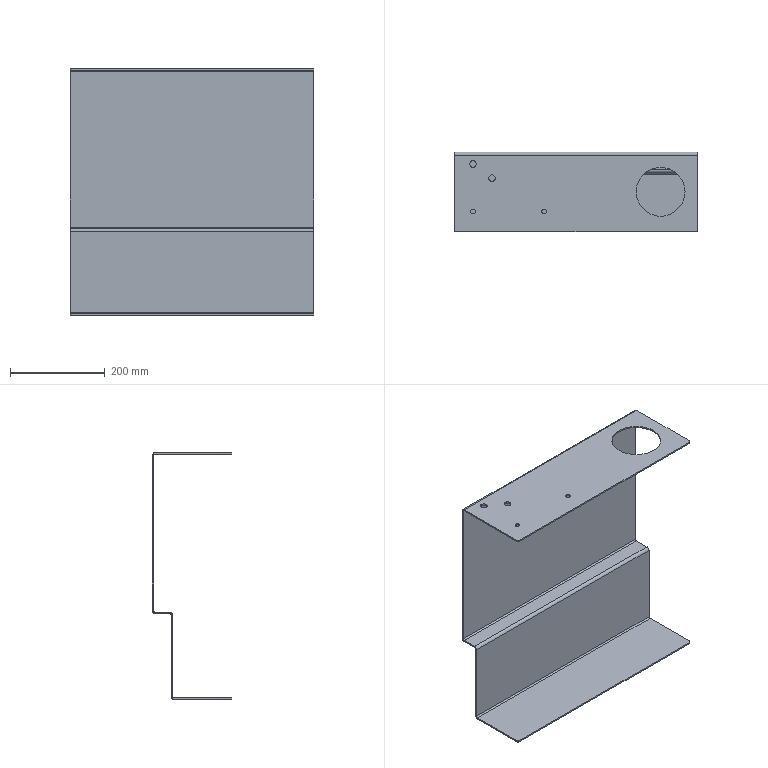Part | SolidWorks | features Fillet 1, FlatPattern 1, ICE 1, SMBaseFlange 1, SheetMetal 1 | 1 solid | 52 faces | box 514 x 167 x 520 mm | volume 1269270 mm3 | plane 30 | cylinder 22 | commonest cylinder face diameters 6 x4 8 x4 10 x4 12 x4 14 x4 103 x2
STEP:
#1=CARTESIAN_POINT('',(487.,83.5,-3.));
#2=VERTEX_POINT('',#1);
#3=CARTESIAN_POINT('',(384.,83.5,-3.));
#4=VERTEX_POINT('',#3);
#5=CARTESIAN_POINT('',(435.5,83.5,-3.));
#6=DIRECTION('',(0.,0.,-1.));
#7=DIRECTION('',(1.,0.,0.));
#8=AXIS2_PLACEMENT_3D('',#5,#6,#7);
#9=CIRCLE('',#8,51.5);
#10=EDGE_CURVE('',#2,#4,#9,.T.);
#11=ORIENTED_EDGE('',*,*,#10,.T.);
#12=CARTESIAN_POINT('',(384.,83.5,0.));
#13=VERTEX_POINT('',#12);
#14=CARTESIAN_POINT('',(384.,83.5,-520.001));
#15=DIRECTION('',(0.,0.,1.));
#16=VECTOR('',#15,1000.);
#17=LINE('',#14,#16);
#18=EDGE_CURVE('',#4,#13,#17,.T.);
#19=ORIENTED_EDGE('',*,*,#18,.T.);
#20=CARTESIAN_POINT('',(487.,83.5,0.));
#21=VERTEX_POINT('',#20);
#22=CARTESIAN_POINT('',(435.5,83.5,0.));
#23=DIRECTION('',(0.,0.,1.));
#24=DIRECTION('',(1.,0.,0.));
#25=AXIS2_PLACEMENT_3D('',#22,#23,#24);
#26=CIRCLE('',#25,51.5);
#27=EDGE_CURVE('',#13,#21,#26,.T.);
#28=ORIENTED_EDGE('',*,*,#27,.T.);
#29=CARTESIAN_POINT('',(487.,83.5,-520.001));
#30=DIRECTION('',(0.,0.,1.));
#31=VECTOR('',#30,1000.);
#32=LINE('',#29,#31);
#33=EDGE_CURVE('',#2,#21,#32,.T.);
#34=ORIENTED_EDGE('',*,*,#33,.F.);
#35=EDGE_LOOP('',(#11,#19,#28,#34));
#36=FACE_OUTER_BOUND('',#35,.T.);
#37=CARTESIAN_POINT('',(435.5,83.5,-520.001));
#38=DIRECTION('',(0.,0.,1.));
#39=DIRECTION('',(1.,0.,0.));
#40=AXIS2_PLACEMENT_3D('',#37,#38,#39);
#41=CYLINDRICAL_SURFACE('',#40,51.5);
#42=ADVANCED_FACE('',(#36),#41,.F.);
#43=CARTESIAN_POINT('',(195.,42.,-3.));
#44=VERTEX_POINT('',#43);
#45=CARTESIAN_POINT('',(185.,42.,-3.));
#46=VERTEX_POINT('',#45);
#47=CARTESIAN_POINT('',(190.,42.,-3.));
#48=DIRECTION('',(0.,0.,-1.));
#49=DIRECTION('',(1.,0.,0.));
#50=AXIS2_PLACEMENT_3D('',#47,#48,#49);
#51=CIRCLE('',#50,5.);
#52=EDGE_CURVE('',#44,#46,#51,.T.);
#53=ORIENTED_EDGE('',*,*,#52,.T.);
#54=CARTESIAN_POINT('',(185.,42.,0.));
#55=VERTEX_POINT('',#54);
#56=CARTESIAN_POINT('',(185.,42.,-520.001));
#57=DIRECTION('',(0.,0.,1.));
#58=VECTOR('',#57,1000.);
#59=LINE('',#56,#58);
#60=EDGE_CURVE('',#46,#55,#59,.T.);
#61=ORIENTED_EDGE('',*,*,#60,.T.);
#62=CARTESIAN_POINT('',(195.,42.,0.));
#63=VERTEX_POINT('',#62);
#64=CARTESIAN_POINT('',(190.,42.,0.));
#65=DIRECTION('',(0.,0.,1.));
#66=DIRECTION('',(1.,0.,0.));
#67=AXIS2_PLACEMENT_3D('',#64,#65,#66);
#68=CIRCLE('',#67,5.);
#69=EDGE_CURVE('',#55,#63,#68,.T.);
#70=ORIENTED_EDGE('',*,*,#69,.T.);
#71=CARTESIAN_POINT('',(195.,42.,-520.001));
#72=DIRECTION('',(0.,0.,1.));
#73=VECTOR('',#72,1000.);
#74=LINE('',#71,#73);
#75=EDGE_CURVE('',#44,#63,#74,.T.);
#76=ORIENTED_EDGE('',*,*,#75,.F.);
#77=EDGE_LOOP('',(#53,#61,#70,#76));
#78=FACE_OUTER_BOUND('',#77,.T.);
#79=CARTESIAN_POINT('',(190.,42.,-520.001));
#80=DIRECTION('',(0.,0.,1.));
#81=DIRECTION('',(1.,0.,0.));
#82=AXIS2_PLACEMENT_3D('',#79,#80,#81);
#83=CYLINDRICAL_SURFACE('',#82,5.);
#84=ADVANCED_FACE('',(#78),#83,.F.);
#85=CARTESIAN_POINT('',(45.,42.,-3.));
#86=VERTEX_POINT('',#85);
#87=CARTESIAN_POINT('',(35.,42.,-3.));
#88=VERTEX_POINT('',#87);
#89=CARTESIAN_POINT('',(40.,42.,-3.));
#90=DIRECTION('',(0.,0.,-1.));
#91=DIRECTION('',(1.,0.,0.));
#92=AXIS2_PLACEMENT_3D('',#89,#90,#91);
#93=CIRCLE('',#92,5.);
#94=EDGE_CURVE('',#86,#88,#93,.T.);
#95=ORIENTED_EDGE('',*,*,#94,.T.);
#96=CARTESIAN_POINT('',(35.,42.,0.));
#97=VERTEX_POINT('',#96);
#98=CARTESIAN_POINT('',(35.,42.,-520.001));
#99=DIRECTION('',(0.,0.,1.));
#100=VECTOR('',#99,1000.);
#101=LINE('',#98,#100);
#102=EDGE_CURVE('',#88,#97,#101,.T.);
#103=ORIENTED_EDGE('',*,*,#102,.T.);
#104=CARTESIAN_POINT('',(45.,42.,0.));
#105=VERTEX_POINT('',#104);
#106=CARTESIAN_POINT('',(40.,42.,0.));
#107=DIRECTION('',(0.,0.,1.));
#108=DIRECTION('',(1.,0.,0.));
#109=AXIS2_PLACEMENT_3D('',#106,#107,#108);
#110=CIRCLE('',#109,5.);
#111=EDGE_CURVE('',#97,#105,#110,.T.);
#112=ORIENTED_EDGE('',*,*,#111,.T.);
#113=CARTESIAN_POINT('',(45.,42.,-520.001));
#114=DIRECTION('',(0.,0.,1.));
#115=VECTOR('',#114,1000.);
#116=LINE('',#113,#115);
#117=EDGE_CURVE('',#86,#105,#116,.T.);
#118=ORIENTED_EDGE('',*,*,#117,.F.);
#119=EDGE_LOOP('',(#95,#103,#112,#118));
#120=FACE_OUTER_BOUND('',#119,.T.);
#121=CARTESIAN_POINT('',(40.,42.,-520.001));
#122=DIRECTION('',(0.,0.,1.));
#123=DIRECTION('',(1.,0.,0.));
#124=AXIS2_PLACEMENT_3D('',#121,#122,#123);
#125=CYLINDRICAL_SURFACE('',#124,5.);
#126=ADVANCED_FACE('',(#120),#125,.F.);
#127=CARTESIAN_POINT('',(87.,112.,-3.));
#128=VERTEX_POINT('',#127);
#129=CARTESIAN_POINT('',(73.,112.,-3.));
#130=VERTEX_POINT('',#129);
#131=CARTESIAN_POINT('',(80.,112.,-3.));
#132=DIRECTION('',(0.,0.,-1.));
#133=DIRECTION('',(1.,0.,0.));
#134=AXIS2_PLACEMENT_3D('',#131,#132,#133);
#135=CIRCLE('',#134,7.);
#136=EDGE_CURVE('',#128,#130,#135,.T.);
#137=ORIENTED_EDGE('',*,*,#136,.T.);
#138=CARTESIAN_POINT('',(73.,112.,0.));
#139=VERTEX_POINT('',#138);
#140=CARTESIAN_POINT('',(73.,112.,-520.001));
#141=DIRECTION('',(0.,0.,1.));
#142=VECTOR('',#141,1000.);
#143=LINE('',#140,#142);
#144=EDGE_CURVE('',#130,#139,#143,.T.);
#145=ORIENTED_EDGE('',*,*,#144,.T.);
#146=CARTESIAN_POINT('',(87.,112.,0.));
#147=VERTEX_POINT('',#146);
#148=CARTESIAN_POINT('',(80.,112.,0.));
#149=DIRECTION('',(0.,0.,1.));
#150=DIRECTION('',(1.,0.,0.));
#151=AXIS2_PLACEMENT_3D('',#148,#149,#150);
#152=CIRCLE('',#151,7.);
#153=EDGE_CURVE('',#139,#147,#152,.T.);
#154=ORIENTED_EDGE('',*,*,#153,.T.);
#155=CARTESIAN_POINT('',(87.,112.,-520.001));
#156=DIRECTION('',(0.,0.,1.));
#157=VECTOR('',#156,1000.);
#158=LINE('',#155,#157);
#159=EDGE_CURVE('',#128,#147,#158,.T.);
#160=ORIENTED_EDGE('',*,*,#159,.F.);
#161=EDGE_LOOP('',(#137,#145,#154,#160));
#162=FACE_OUTER_BOUND('',#161,.T.);
#163=CARTESIAN_POINT('',(80.,112.,-520.001));
#164=DIRECTION('',(0.,0.,1.));
#165=DIRECTION('',(1.,0.,0.));
#166=AXIS2_PLACEMENT_3D('',#163,#164,#165);
#167=CYLINDRICAL_SURFACE('',#166,7.);
#168=ADVANCED_FACE('',(#162),#167,.F.);
#169=CARTESIAN_POINT('',(47.,142.,-3.));
#170=VERTEX_POINT('',#169);
#171=CARTESIAN_POINT('',(33.,142.,-3.));
#172=VERTEX_POINT('',#171);
#173=CARTESIAN_POINT('',(40.,142.,-3.));
#174=DIRECTION('',(0.,0.,-1.));
#175=DIRECTION('',(1.,0.,0.));
#176=AXIS2_PLACEMENT_3D('',#173,#174,#175);
#177=CIRCLE('',#176,7.);
#178=EDGE_CURVE('',#170,#172,#177,.T.);
#179=ORIENTED_EDGE('',*,*,#178,.T.);
#180=CARTESIAN_POINT('',(33.,142.,0.));
#181=VERTEX_POINT('',#180);
#182=CARTESIAN_POINT('',(33.,142.,-520.001));
#183=DIRECTION('',(0.,0.,1.));
#184=VECTOR('',#183,1000.);
#185=LINE('',#182,#184);
#186=EDGE_CURVE('',#172,#181,#185,.T.);
#187=ORIENTED_EDGE('',*,*,#186,.T.);
#188=CARTESIAN_POINT('',(47.,142.,0.));
#189=VERTEX_POINT('',#188);
#190=CARTESIAN_POINT('',(40.,142.,0.));
#191=DIRECTION('',(0.,0.,1.));
#192=DIRECTION('',(1.,0.,0.));
#193=AXIS2_PLACEMENT_3D('',#190,#191,#192);
#194=CIRCLE('',#193,7.);
#195=EDGE_CURVE('',#181,#189,#194,.T.);
#196=ORIENTED_EDGE('',*,*,#195,.T.);
#197=CARTESIAN_POINT('',(47.,142.,-520.001));
#198=DIRECTION('',(0.,0.,1.));
#199=VECTOR('',#198,1000.);
#200=LINE('',#197,#199);
#201=EDGE_CURVE('',#170,#189,#200,.T.);
#202=ORIENTED_EDGE('',*,*,#201,.F.);
#203=EDGE_LOOP('',(#179,#187,#196,#202));
#204=FACE_OUTER_BOUND('',#203,.T.);
#205=CARTESIAN_POINT('',(40.,142.,-520.001));
#206=DIRECTION('',(0.,0.,1.));
#207=DIRECTION('',(1.,0.,0.));
#208=AXIS2_PLACEMENT_3D('',#205,#206,#207);
#209=CYLINDRICAL_SURFACE('',#208,7.);
#210=ADVANCED_FACE('',(#204),#209,.F.);
#211=CARTESIAN_POINT('',(514.,167.,-6.));
#212=VERTEX_POINT('',#211);
#213=CARTESIAN_POINT('',(514.,164.,-6.));
#214=VERTEX_POINT('',#213);
#215=CARTESIAN_POINT('',(514.,167.,-6.));
#216=DIRECTION('',(0.,-1.,0.));
#217=VECTOR('',#216,1000.);
#218=LINE('',#215,#217);
#219=EDGE_CURVE('',#212,#214,#218,.T.);
#220=ORIENTED_EDGE('',*,*,#219,.F.);
#221=CARTESIAN_POINT('',(514.,161.,0.));
#222=VERTEX_POINT('',#221);
#223=CARTESIAN_POINT('',(514.,161.,-6.));
#224=DIRECTION('',(-1.,0.,0.));
#225=DIRECTION('',(0.,0.,-1.));
#226=AXIS2_PLACEMENT_3D('',#223,#224,#225);
#227=CIRCLE('',#226,6.);
#228=EDGE_CURVE('',#222,#212,#227,.T.);
#229=ORIENTED_EDGE('',*,*,#228,.F.);
#230=CARTESIAN_POINT('',(514.,161.,-3.));
#231=VERTEX_POINT('',#230);
#232=CARTESIAN_POINT('',(514.,161.,-3.));
#233=DIRECTION('',(0.,0.,1.));
#234=VECTOR('',#233,1000.);
#235=LINE('',#232,#234);
#236=EDGE_CURVE('',#231,#222,#235,.T.);
#237=ORIENTED_EDGE('',*,*,#236,.F.);
#238=CARTESIAN_POINT('',(514.,161.,-6.));
#239=DIRECTION('',(-1.,0.,0.));
#240=DIRECTION('',(0.,0.,-1.));
#241=AXIS2_PLACEMENT_3D('',#238,#239,#240);
#242=CIRCLE('',#241,3.);
#243=EDGE_CURVE('',#231,#214,#242,.T.);
#244=ORIENTED_EDGE('',*,*,#243,.T.);
#245=EDGE_LOOP('',(#220,#229,#237,#244));
#246=FACE_OUTER_BOUND('',#245,.T.);
#247=CARTESIAN_POINT('',(514.,167.,-6.));
#248=DIRECTION('',(1.,0.,0.));
#249=DIRECTION('',(0.,0.,-1.));
#250=AXIS2_PLACEMENT_3D('',#247,#248,#249);
#251=PLANE('',#250);
#252=ADVANCED_FACE('',(#246),#251,.T.);
#253=CARTESIAN_POINT('',(514.,167.,-334.));
#254=VERTEX_POINT('',#253);
#255=CARTESIAN_POINT('',(514.,167.,0.));
#256=DIRECTION('',(0.,0.,-1.));
#257=VECTOR('',#256,1000.);
#258=LINE('',#255,#257);
#259=EDGE_CURVE('',#212,#254,#258,.T.);
#260=ORIENTED_EDGE('',*,*,#259,.F.);
#261=ORIENTED_EDGE('',*,*,#219,.T.);
#262=CARTESIAN_POINT('',(514.,164.,-334.));
#263=VERTEX_POINT('',#262);
#264=CARTESIAN_POINT('',(514.,164.,0.));
#265=DIRECTION('',(0.,0.,-1.));
#266=VECTOR('',#265,1000.);
#267=LINE('',#264,#266);
#268=EDGE_CURVE('',#214,#263,#267,.T.);
#269=ORIENTED_EDGE('',*,*,#268,.T.);
#270=CARTESIAN_POINT('',(514.,164.,-334.));
#271=DIRECTION('',(0.,1.,0.));
#272=VECTOR('',#271,1000.);
#273=LINE('',#270,#272);
#274=EDGE_CURVE('',#263,#254,#273,.T.);
#275=ORIENTED_EDGE('',*,*,#274,.T.);
#276=EDGE_LOOP('',(#260,#261,#269,#275));
#277=FACE_OUTER_BOUND('',#276,.T.);
#278=CARTESIAN_POINT('',(514.,161.,-3.));
#279=DIRECTION('',(1.,0.,0.));
#280=DIRECTION('',(0.,0.,-1.));
#281=AXIS2_PLACEMENT_3D('',#278,#279,#280);
#282=PLANE('',#281);
#283=ADVANCED_FACE('',(#277),#282,.T.);
#284=CARTESIAN_POINT('',(0.,161.,0.));
#285=VERTEX_POINT('',#284);
#286=CARTESIAN_POINT('',(0.,161.,-3.));
#287=VERTEX_POINT('',#286);
#288=CARTESIAN_POINT('',(0.,161.,0.));
#289=DIRECTION('',(0.,0.,-1.));
#290=VECTOR('',#289,1000.);
#291=LINE('',#288,#290);
#292=EDGE_CURVE('',#285,#287,#291,.T.);
#293=ORIENTED_EDGE('',*,*,#292,.F.);
#294=CARTESIAN_POINT('',(0.,167.,-6.));
#295=VERTEX_POINT('',#294);
#296=CARTESIAN_POINT('',(0.,161.,-6.));
#297=DIRECTION('',(-1.,0.,0.));
#298=DIRECTION('',(0.,0.,-1.));
#299=AXIS2_PLACEMENT_3D('',#296,#297,#298);
#300=CIRCLE('',#299,6.);
#301=EDGE_CURVE('',#285,#295,#300,.T.);
#302=ORIENTED_EDGE('',*,*,#301,.T.);
#303=CARTESIAN_POINT('',(0.,164.,-6.));
#304=VERTEX_POINT('',#303);
#305=CARTESIAN_POINT('',(0.,164.,-6.));
#306=DIRECTION('',(0.,1.,0.));
#307=VECTOR('',#306,1000.);
#308=LINE('',#305,#307);
#309=EDGE_CURVE('',#304,#295,#308,.T.);
#310=ORIENTED_EDGE('',*,*,#309,.F.);
#311=CARTESIAN_POINT('',(0.,161.,-6.));
#312=DIRECTION('',(-1.,0.,0.));
#313=DIRECTION('',(0.,0.,-1.));
#314=AXIS2_PLACEMENT_3D('',#311,#312,#313);
#315=CIRCLE('',#314,3.);
#316=EDGE_CURVE('',#287,#304,#315,.T.);
#317=ORIENTED_EDGE('',*,*,#316,.F.);
#318=EDGE_LOOP('',(#293,#302,#310,#317));
#319=FACE_OUTER_BOUND('',#318,.T.);
#320=CARTESIAN_POINT('',(0.,161.,0.));
#321=DIRECTION('',(-1.,0.,0.));
#322=DIRECTION('',(0.,0.,1.));
#323=AXIS2_PLACEMENT_3D('',#320,#321,#322);
#324=PLANE('',#323);
#325=ADVANCED_FACE('',(#319),#324,.T.);
#326=CARTESIAN_POINT('',(0.,4.,-3.));
#327=VERTEX_POINT('',#326);
#328=CARTESIAN_POINT('',(0.,0.,-3.));
#329=DIRECTION('',(0.,1.,0.));
#330=VECTOR('',#329,1000.);
#331=LINE('',#328,#330);
#332=EDGE_CURVE('',#327,#287,#331,.T.);
#333=ORIENTED_EDGE('',*,*,#332,.F.);
#334=CARTESIAN_POINT('',(0.,4.,0.));
#335=VERTEX_POINT('',#334);
#336=CARTESIAN_POINT('',(0.,4.,-6.));
#337=DIRECTION('',(0.,0.,1.));
#338=VECTOR('',#337,1000.);
#339=LINE('',#336,#338);
#340=EDGE_CURVE('',#327,#335,#339,.T.);
#341=ORIENTED_EDGE('',*,*,#340,.T.);
#342=CARTESIAN_POINT('',(0.,0.,0.));
#343=DIRECTION('',(0.,1.,0.));
#344=VECTOR('',#343,1000.);
#345=LINE('',#342,#344);
#346=EDGE_CURVE('',#335,#285,#345,.T.);
#347=ORIENTED_EDGE('',*,*,#346,.T.);
#348=ORIENTED_EDGE('',*,*,#292,.T.);
#349=EDGE_LOOP('',(#333,#341,#347,#348));
#350=FACE_OUTER_BOUND('',#349,.T.);
#351=CARTESIAN_POINT('',(0.,164.,-6.));
#352=DIRECTION('',(-1.,0.,0.));
#353=DIRECTION('',(0.,0.,1.));
#354=AXIS2_PLACEMENT_3D('',#351,#352,#353);
#355=PLANE('',#354);
#356=ADVANCED_FACE('',(#350),#355,.T.);
#357=CARTESIAN_POINT('',(514.,161.,-340.));
#358=VERTEX_POINT('',#357);
#359=CARTESIAN_POINT('',(514.,161.,-337.));
#360=VERTEX_POINT('',#359);
#361=CARTESIAN_POINT('',(514.,161.,-340.));
#362=DIRECTION('',(0.,0.,1.));
#363=VECTOR('',#362,1000.);
#364=LINE('',#361,#363);
#365=EDGE_CURVE('',#358,#360,#364,.T.);
#366=ORIENTED_EDGE('',*,*,#365,.F.);
#367=CARTESIAN_POINT('',(514.,161.,-334.));
#368=DIRECTION('',(-1.,0.,0.));
#369=DIRECTION('',(0.,0.,-1.));
#370=AXIS2_PLACEMENT_3D('',#367,#368,#369);
#371=CIRCLE('',#370,6.);
#372=EDGE_CURVE('',#254,#358,#371,.T.);
#373=ORIENTED_EDGE('',*,*,#372,.F.);
#374=ORIENTED_EDGE('',*,*,#274,.F.);
#375=CARTESIAN_POINT('',(514.,161.,-334.));
#376=DIRECTION('',(-1.,0.,0.));
#377=DIRECTION('',(0.,0.,-1.));
#378=AXIS2_PLACEMENT_3D('',#375,#376,#377);
#379=CIRCLE('',#378,3.);
#380=EDGE_CURVE('',#263,#360,#379,.T.);
#381=ORIENTED_EDGE('',*,*,#380,.T.);
#382=EDGE_LOOP('',(#366,#373,#374,#381));
#383=FACE_OUTER_BOUND('',#382,.T.);
#384=CARTESIAN_POINT('',(514.,161.,-340.));
#385=DIRECTION('',(1.,0.,0.));
#386=DIRECTION('',(0.,0.,-1.));
#387=AXIS2_PLACEMENT_3D('',#384,#385,#386);
#388=PLANE('',#387);
#389=ADVANCED_FACE('',(#383),#388,.T.);
#390=CARTESIAN_POINT('',(514.,130.,-340.));
#391=VERTEX_POINT('',#390);
#392=CARTESIAN_POINT('',(514.,167.,-340.));
#393=DIRECTION('',(0.,-1.,0.));
#394=VECTOR('',#393,1000.);
#395=LINE('',#392,#394);
#396=EDGE_CURVE('',#358,#391,#395,.T.);
#397=ORIENTED_EDGE('',*,*,#396,.F.);
#398=ORIENTED_EDGE('',*,*,#365,.T.);
#399=CARTESIAN_POINT('',(514.,130.,-337.));
#400=VERTEX_POINT('',#399);
#401=CARTESIAN_POINT('',(514.,167.,-337.));
#402=DIRECTION('',(0.,-1.,0.));
#403=VECTOR('',#402,1000.);
#404=LINE('',#401,#403);
#405=EDGE_CURVE('',#360,#400,#404,.T.);
#406=ORIENTED_EDGE('',*,*,#405,.T.);
#407=CARTESIAN_POINT('',(514.,130.,-337.));
#408=DIRECTION('',(0.,0.,-1.));
#409=VECTOR('',#408,1000.);
#410=LINE('',#407,#409);
#411=EDGE_CURVE('',#400,#391,#410,.T.);
#412=ORIENTED_EDGE('',*,*,#411,.T.);
#413=EDGE_LOOP('',(#397,#398,#406,#412));
#414=FACE_OUTER_BOUND('',#413,.T.);
#415=CARTESIAN_POINT('',(514.,164.,-334.));
#416=DIRECTION('',(1.,0.,0.));
#417=DIRECTION('',(0.,0.,-1.));
#418=AXIS2_PLACEMENT_3D('',#415,#416,#417);
#419=PLANE('',#418);
#420=ADVANCED_FACE('',(#414),#419,.T.);
#421=CARTESIAN_POINT('',(0.,167.,-334.));
#422=VERTEX_POINT('',#421);
#423=CARTESIAN_POINT('',(0.,164.,-334.));
#424=VERTEX_POINT('',#423);
#425=CARTESIAN_POINT('',(0.,167.,-334.));
#426=DIRECTION('',(0.,-1.,0.));
#427=VECTOR('',#426,1000.);
#428=LINE('',#425,#427);
#429=EDGE_CURVE('',#422,#424,#428,.T.);
#430=ORIENTED_EDGE('',*,*,#429,.F.);
#431=CARTESIAN_POINT('',(0.,161.,-340.));
#432=VERTEX_POINT('',#431);
#433=CARTESIAN_POINT('',(0.,161.,-334.));
#434=DIRECTION('',(-1.,0.,0.));
#435=DIRECTION('',(0.,0.,-1.));
#436=AXIS2_PLACEMENT_3D('',#433,#434,#435);
#437=CIRCLE('',#436,6.);
#438=EDGE_CURVE('',#422,#432,#437,.T.);
#439=ORIENTED_EDGE('',*,*,#438,.T.);
#440=CARTESIAN_POINT('',(0.,161.,-337.));
#441=VERTEX_POINT('',#440);
#442=CARTESIAN_POINT('',(0.,161.,-337.));
#443=DIRECTION('',(0.,0.,-1.));
#444=VECTOR('',#443,1000.);
#445=LINE('',#442,#444);
#446=EDGE_CURVE('',#441,#432,#445,.T.);
#447=ORIENTED_EDGE('',*,*,#446,.F.);
#448=CARTESIAN_POINT('',(0.,161.,-334.));
#449=DIRECTION('',(-1.,0.,0.));
#450=DIRECTION('',(0.,0.,-1.));
#451=AXIS2_PLACEMENT_3D('',#448,#449,#450);
#452=CIRCLE('',#451,3.);
#453=EDGE_CURVE('',#424,#441,#452,.T.);
#454=ORIENTED_EDGE('',*,*,#453,.F.);
#455=EDGE_LOOP('',(#430,#439,#447,#454));
#456=FACE_OUTER_BOUND('',#455,.T.);
#457=CARTESIAN_POINT('',(0.,167.,-334.));
#458=DIRECTION('',(-1.,0.,0.));
#459=DIRECTION('',(0.,0.,1.));
#460=AXIS2_PLACEMENT_3D('',#457,#458,#459);
#461=PLANE('',#460);
#462=ADVANCED_FACE('',(#456),#461,.T.);
#463=CARTESIAN_POINT('',(0.,167.,0.));
#464=DIRECTION('',(0.,0.,-1.));
#465=VECTOR('',#464,1000.);
#466=LINE('',#463,#465);
#467=EDGE_CURVE('',#295,#422,#466,.T.);
#468=ORIENTED_EDGE('',*,*,#467,.T.);
#469=ORIENTED_EDGE('',*,*,#429,.T.);
#470=CARTESIAN_POINT('',(0.,164.,0.));
#471=DIRECTION('',(0.,0.,-1.));
#472=VECTOR('',#471,1000.);
#473=LINE('',#470,#472);
#474=EDGE_CURVE('',#304,#424,#473,.T.);
#475=ORIENTED_EDGE('',*,*,#474,.F.);
#476=ORIENTED_EDGE('',*,*,#309,.T.);
#477=EDGE_LOOP('',(#468,#469,#475,#476));
#478=FACE_OUTER_BOUND('',#477,.T.);
#479=CARTESIAN_POINT('',(0.,161.,-337.));
#480=DIRECTION('',(-1.,0.,0.));
#481=DIRECTION('',(0.,0.,1.));
#482=AXIS2_PLACEMENT_3D('',#479,#480,#481);
#483=PLANE('',#482);
#484=ADVANCED_FACE('',(#478),#483,.T.);
#485=CARTESIAN_POINT('',(514.,127.,-343.));
#486=VERTEX_POINT('',#485);
#487=CARTESIAN_POINT('',(514.,124.,-343.));
#488=VERTEX_POINT('',#487);
#489=CARTESIAN_POINT('',(514.,127.,-343.));
#490=DIRECTION('',(0.,-1.,0.));
#491=VECTOR('',#490,1000.);
#492=LINE('',#489,#491);
#493=EDGE_CURVE('',#486,#488,#492,.T.);
#494=ORIENTED_EDGE('',*,*,#493,.F.);
#495=CARTESIAN_POINT('',(514.,130.,-343.));
#496=DIRECTION('',(1.,0.,0.));
#497=DIRECTION('',(0.,0.,1.));
#498=AXIS2_PLACEMENT_3D('',#495,#496,#497);
#499=CIRCLE('',#498,3.);
#500=EDGE_CURVE('',#391,#486,#499,.T.);
#501=ORIENTED_EDGE('',*,*,#500,.F.);
#502=ORIENTED_EDGE('',*,*,#411,.F.);
#503=CARTESIAN_POINT('',(514.,130.,-343.));
#504=DIRECTION('',(1.,0.,0.));
#505=DIRECTION('',(0.,0.,-1.));
#506=AXIS2_PLACEMENT_3D('',#503,#504,#505);
#507=CIRCLE('',#506,6.);
#508=EDGE_CURVE('',#400,#488,#507,.T.);
#509=ORIENTED_EDGE('',*,*,#508,.T.);
#510=EDGE_LOOP('',(#494,#501,#502,#509));
#511=FACE_OUTER_BOUND('',#510,.T.);
#512=CARTESIAN_POINT('',(514.,127.,-343.));
#513=DIRECTION('',(1.,0.,0.));
#514=DIRECTION('',(0.,0.,-1.));
#515=AXIS2_PLACEMENT_3D('',#512,#513,#514);
#516=PLANE('',#515);
#517=ADVANCED_FACE('',(#511),#516,.T.);
#518=CARTESIAN_POINT('',(514.,127.,-514.));
#519=VERTEX_POINT('',#518);
#520=CARTESIAN_POINT('',(514.,127.,-340.));
#521=DIRECTION('',(0.,0.,-1.));
#522=VECTOR('',#521,1000.);
#523=LINE('',#520,#522);
#524=EDGE_CURVE('',#486,#519,#523,.T.);
#525=ORIENTED_EDGE('',*,*,#524,.F.);
#526=ORIENTED_EDGE('',*,*,#493,.T.);
#527=CARTESIAN_POINT('',(514.,124.,-514.));
#528=VERTEX_POINT('',#527);
#529=CARTESIAN_POINT('',(514.,124.,-340.));
#530=DIRECTION('',(0.,0.,-1.));
#531=VECTOR('',#530,1000.);
#532=LINE('',#529,#531);
#533=EDGE_CURVE('',#488,#528,#532,.T.);
#534=ORIENTED_EDGE('',*,*,#533,.T.);
#535=CARTESIAN_POINT('',(514.,124.,-514.));
#536=DIRECTION('',(0.,1.,0.));
#537=VECTOR('',#536,1000.);
#538=LINE('',#535,#537);
#539=EDGE_CURVE('',#528,#519,#538,.T.);
#540=ORIENTED_EDGE('',*,*,#539,.T.);
#541=EDGE_LOOP('',(#525,#526,#534,#540));
#542=FACE_OUTER_BOUND('',#541,.T.);
#543=CARTESIAN_POINT('',(514.,130.,-337.));
#544=DIRECTION('',(1.,0.,0.));
#545=DIRECTION('',(0.,0.,-1.));
#546=AXIS2_PLACEMENT_3D('',#543,#544,#545);
#547=PLANE('',#546);
#548=ADVANCED_FACE('',(#542),#547,.T.);
#549=CARTESIAN_POINT('',(0.,130.,-340.));
#550=VERTEX_POINT('',#549);
#551=CARTESIAN_POINT('',(0.,130.,-337.));
#552=VERTEX_POINT('',#551);
#553=CARTESIAN_POINT('',(0.,130.,-340.));
#554=DIRECTION('',(0.,0.,1.));
#555=VECTOR('',#554,1000.);
#556=LINE('',#553,#555);
#557=EDGE_CURVE('',#550,#552,#556,.T.);
#558=ORIENTED_EDGE('',*,*,#557,.F.);
#559=CARTESIAN_POINT('',(0.,127.,-343.));
#560=VERTEX_POINT('',#559);
#561=CARTESIAN_POINT('',(0.,130.,-343.));
#562=DIRECTION('',(1.,0.,0.));
#563=DIRECTION('',(0.,0.,1.));
#564=AXIS2_PLACEMENT_3D('',#561,#562,#563);
#565=CIRCLE('',#564,3.);
#566=EDGE_CURVE('',#550,#560,#565,.T.);
#567=ORIENTED_EDGE('',*,*,#566,.T.);
#568=CARTESIAN_POINT('',(0.,124.,-343.));
#569=VERTEX_POINT('',#568);
#570=CARTESIAN_POINT('',(0.,124.,-343.));
#571=DIRECTION('',(0.,1.,0.));
#572=VECTOR('',#571,1000.);
#573=LINE('',#570,#572);
#574=EDGE_CURVE('',#569,#560,#573,.T.);
#575=ORIENTED_EDGE('',*,*,#574,.F.);
#576=CARTESIAN_POINT('',(0.,130.,-343.));
#577=DIRECTION('',(1.,0.,0.));
#578=DIRECTION('',(0.,0.,-1.));
#579=AXIS2_PLACEMENT_3D('',#576,#577,#578);
#580=CIRCLE('',#579,6.);
#581=EDGE_CURVE('',#552,#569,#580,.T.);
#582=ORIENTED_EDGE('',*,*,#581,.F.);
#583=EDGE_LOOP('',(#558,#567,#575,#582));
#584=FACE_OUTER_BOUND('',#583,.T.);
#585=CARTESIAN_POINT('',(0.,130.,-340.));
#586=DIRECTION('',(-1.,0.,0.));
#587=DIRECTION('',(0.,0.,1.));
#588=AXIS2_PLACEMENT_3D('',#585,#586,#587);
#589=PLANE('',#588);
#590=ADVANCED_FACE('',(#584),#589,.T.);
#591=CARTESIAN_POINT('',(0.,167.,-340.));
#592=DIRECTION('',(0.,-1.,0.));
#593=VECTOR('',#592,1000.);
#594=LINE('',#591,#593);
#595=EDGE_CURVE('',#432,#550,#594,.T.);
#596=ORIENTED_EDGE('',*,*,#595,.T.);
#597=ORIENTED_EDGE('',*,*,#557,.T.);
#598=CARTESIAN_POINT('',(0.,167.,-337.));
#599=DIRECTION('',(0.,-1.,0.));
#600=VECTOR('',#599,1000.);
#601=LINE('',#598,#600);
#602=EDGE_CURVE('',#441,#552,#601,.T.);
#603=ORIENTED_EDGE('',*,*,#602,.F.);
#604=ORIENTED_EDGE('',*,*,#446,.T.);
#605=EDGE_LOOP('',(#596,#597,#603,#604));
#606=FACE_OUTER_BOUND('',#605,.T.);
#607=CARTESIAN_POINT('',(0.,124.,-343.));
#608=DIRECTION('',(-1.,0.,0.));
#609=DIRECTION('',(0.,0.,1.));
#610=AXIS2_PLACEMENT_3D('',#607,#608,#609);
#611=PLANE('',#610);
#612=ADVANCED_FACE('',(#606),#611,.T.);
#613=CARTESIAN_POINT('',(514.,121.,-520.));
#614=VERTEX_POINT('',#613);
#615=CARTESIAN_POINT('',(514.,121.,-517.));
#616=VERTEX_POINT('',#615);
#617=CARTESIAN_POINT('',(514.,121.,-520.));
#618=DIRECTION('',(0.,0.,1.));
#619=VECTOR('',#618,1000.);
#620=LINE('',#617,#619);
#621=EDGE_CURVE('',#614,#616,#620,.T.);
#622=ORIENTED_EDGE('',*,*,#621,.F.);
#623=CARTESIAN_POINT('',(514.,121.,-514.));
#624=DIRECTION('',(-1.,0.,0.));
#625=DIRECTION('',(0.,0.,-1.));
#626=AXIS2_PLACEMENT_3D('',#623,#624,#625);
#627=CIRCLE('',#626,6.);
#628=EDGE_CURVE('',#519,#614,#627,.T.);
#629=ORIENTED_EDGE('',*,*,#628,.F.);
#630=ORIENTED_EDGE('',*,*,#539,.F.);
#631=CARTESIAN_POINT('',(514.,121.,-514.));
#632=DIRECTION('',(-1.,0.,0.));
#633=DIRECTION('',(0.,0.,-1.));
#634=AXIS2_PLACEMENT_3D('',#631,#632,#633);
#635=CIRCLE('',#634,3.);
#636=EDGE_CURVE('',#528,#616,#635,.T.);
#637=ORIENTED_EDGE('',*,*,#636,.T.);
#638=EDGE_LOOP('',(#622,#629,#630,#637));
#639=FACE_OUTER_BOUND('',#638,.T.);
#640=CARTESIAN_POINT('',(514.,121.,-520.));
#641=DIRECTION('',(1.,0.,0.));
#642=DIRECTION('',(0.,0.,-1.));
#643=AXIS2_PLACEMENT_3D('',#640,#641,#642);
#644=PLANE('',#643);
#645=ADVANCED_FACE('',(#639),#644,.T.);
#646=CARTESIAN_POINT('',(514.,4.,-517.));
#647=VERTEX_POINT('',#646);
#648=CARTESIAN_POINT('',(514.,127.,-517.));
#649=DIRECTION('',(0.,-1.,0.));
#650=VECTOR('',#649,1000.);
#651=LINE('',#648,#650);
#652=EDGE_CURVE('',#616,#647,#651,.T.);
#653=ORIENTED_EDGE('',*,*,#652,.T.);
#654=CARTESIAN_POINT('',(514.,4.,-520.));
#655=VERTEX_POINT('',#654);
#656=CARTESIAN_POINT('',(514.,4.,-514.));
#657=DIRECTION('',(0.,0.,-1.));
#658=VECTOR('',#657,1000.);
#659=LINE('',#656,#658);
#660=EDGE_CURVE('',#647,#655,#659,.T.);
#661=ORIENTED_EDGE('',*,*,#660,.T.);
#662=CARTESIAN_POINT('',(514.,127.,-520.));
#663=DIRECTION('',(0.,-1.,0.));
#664=VECTOR('',#663,1000.);
#665=LINE('',#662,#664);
#666=EDGE_CURVE('',#614,#655,#665,.T.);
#667=ORIENTED_EDGE('',*,*,#666,.F.);
#668=ORIENTED_EDGE('',*,*,#621,.T.);
#669=EDGE_LOOP('',(#653,#661,#667,#668));
#670=FACE_OUTER_BOUND('',#669,.T.);
#671=CARTESIAN_POINT('',(514.,124.,-514.));
#672=DIRECTION('',(1.,0.,0.));
#673=DIRECTION('',(0.,0.,-1.));
#674=AXIS2_PLACEMENT_3D('',#671,#672,#673);
#675=PLANE('',#674);
#676=ADVANCED_FACE('',(#670),#675,.T.);
#677=CARTESIAN_POINT('',(0.,127.,-514.));
#678=VERTEX_POINT('',#677);
#679=CARTESIAN_POINT('',(0.,124.,-514.));
#680=VERTEX_POINT('',#679);
#681=CARTESIAN_POINT('',(0.,127.,-514.));
#682=DIRECTION('',(0.,-1.,0.));
#683=VECTOR('',#682,1000.);
#684=LINE('',#681,#683);
#685=EDGE_CURVE('',#678,#680,#684,.T.);
#686=ORIENTED_EDGE('',*,*,#685,.F.);
#687=CARTESIAN_POINT('',(0.,121.,-520.));
#688=VERTEX_POINT('',#687);
#689=CARTESIAN_POINT('',(0.,121.,-514.));
#690=DIRECTION('',(-1.,0.,0.));
#691=DIRECTION('',(0.,0.,-1.));
#692=AXIS2_PLACEMENT_3D('',#689,#690,#691);
#693=CIRCLE('',#692,6.);
#694=EDGE_CURVE('',#678,#688,#693,.T.);
#695=ORIENTED_EDGE('',*,*,#694,.T.);
#696=CARTESIAN_POINT('',(0.,121.,-517.));
#697=VERTEX_POINT('',#696);
#698=CARTESIAN_POINT('',(0.,121.,-517.));
#699=DIRECTION('',(0.,0.,-1.));
#700=VECTOR('',#699,1000.);
#701=LINE('',#698,#700);
#702=EDGE_CURVE('',#697,#688,#701,.T.);
#703=ORIENTED_EDGE('',*,*,#702,.F.);
#704=CARTESIAN_POINT('',(0.,121.,-514.));
#705=DIRECTION('',(-1.,0.,0.));
#706=DIRECTION('',(0.,0.,-1.));
#707=AXIS2_PLACEMENT_3D('',#704,#705,#706);
#708=CIRCLE('',#707,3.);
#709=EDGE_CURVE('',#680,#697,#708,.T.);
#710=ORIENTED_EDGE('',*,*,#709,.F.);
#711=EDGE_LOOP('',(#686,#695,#703,#710));
#712=FACE_OUTER_BOUND('',#711,.T.);
#713=CARTESIAN_POINT('',(0.,127.,-514.));
#714=DIRECTION('',(-1.,0.,0.));
#715=DIRECTION('',(0.,0.,1.));
#716=AXIS2_PLACEMENT_3D('',#713,#714,#715);
#717=PLANE('',#716);
#718=ADVANCED_FACE('',(#712),#717,.T.);
#719=CARTESIAN_POINT('',(0.,127.,-340.));
#720=DIRECTION('',(0.,0.,-1.));
#721=VECTOR('',#720,1000.);
#722=LINE('',#719,#721);
#723=EDGE_CURVE('',#560,#678,#722,.T.);
#724=ORIENTED_EDGE('',*,*,#723,.T.);
#725=ORIENTED_EDGE('',*,*,#685,.T.);
#726=CARTESIAN_POINT('',(0.,124.,-340.));
#727=DIRECTION('',(0.,0.,-1.));
#728=VECTOR('',#727,1000.);
#729=LINE('',#726,#728);
#730=EDGE_CURVE('',#569,#680,#729,.T.);
#731=ORIENTED_EDGE('',*,*,#730,.F.);
#732=ORIENTED_EDGE('',*,*,#574,.T.);
#733=EDGE_LOOP('',(#724,#725,#731,#732));
#734=FACE_OUTER_BOUND('',#733,.T.);
#735=CARTESIAN_POINT('',(0.,121.,-517.));
#736=DIRECTION('',(-1.,0.,0.));
#737=DIRECTION('',(0.,0.,1.));
#738=AXIS2_PLACEMENT_3D('',#735,#736,#737);
#739=PLANE('',#738);
#740=ADVANCED_FACE('',(#734),#739,.T.);
#741=CARTESIAN_POINT('',(0.,4.,-517.));
#742=VERTEX_POINT('',#741);
#743=CARTESIAN_POINT('',(0.,127.,-517.));
#744=DIRECTION('',(0.,-1.,0.));
#745=VECTOR('',#744,1000.);
#746=LINE('',#743,#745);
#747=EDGE_CURVE('',#697,#742,#746,.T.);
#748=ORIENTED_EDGE('',*,*,#747,.T.);
#749=CARTESIAN_POINT('',(4.,0.,-517.));
#750=VERTEX_POINT('',#749);
#751=CARTESIAN_POINT('',(4.,4.,-517.));
#752=DIRECTION('',(0.,0.,1.));
#753=DIRECTION('',(-1.,0.,0.));
#754=AXIS2_PLACEMENT_3D('',#751,#752,#753);
#755=CIRCLE('',#754,4.);
#756=EDGE_CURVE('',#742,#750,#755,.T.);
#757=ORIENTED_EDGE('',*,*,#756,.T.);
#758=CARTESIAN_POINT('',(510.,0.,-517.));
#759=VERTEX_POINT('',#758);
#760=CARTESIAN_POINT('',(514.,0.,-517.));
#761=DIRECTION('',(-1.,0.,0.));
#762=VECTOR('',#761,1000.);
#763=LINE('',#760,#762);
#764=EDGE_CURVE('',#759,#750,#763,.T.);
#765=ORIENTED_EDGE('',*,*,#764,.F.);
#766=CARTESIAN_POINT('',(510.,4.,-517.));
#767=DIRECTION('',(0.,0.,1.));
#768=DIRECTION('',(-1.,0.,0.));
#769=AXIS2_PLACEMENT_3D('',#766,#767,#768);
#770=CIRCLE('',#769,4.);
#771=EDGE_CURVE('',#759,#647,#770,.T.);
#772=ORIENTED_EDGE('',*,*,#771,.T.);
#773=ORIENTED_EDGE('',*,*,#652,.F.);
#774=CARTESIAN_POINT('',(514.,121.,-517.));
#775=DIRECTION('',(-1.,0.,0.));
#776=VECTOR('',#775,1000.);
#777=LINE('',#774,#776);
#778=EDGE_CURVE('',#616,#697,#777,.T.);
#779=ORIENTED_EDGE('',*,*,#778,.T.);
#780=EDGE_LOOP('',(#748,#757,#765,#772,#773,#779));
#781=FACE_OUTER_BOUND('',#780,.T.);
#782=CARTESIAN_POINT('',(514.,127.,-517.));
#783=DIRECTION('',(0.,0.,-1.));
#784=DIRECTION('',(-1.,0.,0.));
#785=AXIS2_PLACEMENT_3D('',#782,#783,#784);
#786=PLANE('',#785);
#787=ADVANCED_FACE('',(#781),#786,.F.);
#788=ORIENTED_EDGE('',*,*,#764,.T.);
#789=CARTESIAN_POINT('',(4.,0.,-520.));
#790=VERTEX_POINT('',#789);
#791=CARTESIAN_POINT('',(4.,0.,-520.));
#792=DIRECTION('',(0.,0.,-1.));
#793=VECTOR('',#792,1000.);
#794=LINE('',#791,#793);
#795=EDGE_CURVE('',#750,#790,#794,.T.);
#796=ORIENTED_EDGE('',*,*,#795,.T.);
#797=CARTESIAN_POINT('',(510.,0.,-520.));
#798=VERTEX_POINT('',#797);
#799=CARTESIAN_POINT('',(514.,0.,-520.));
#800=DIRECTION('',(-1.,0.,0.));
#801=VECTOR('',#800,1000.);
#802=LINE('',#799,#801);
#803=EDGE_CURVE('',#798,#790,#802,.T.);
#804=ORIENTED_EDGE('',*,*,#803,.F.);
#805=CARTESIAN_POINT('',(510.,0.,-520.));
#806=DIRECTION('',(0.,0.,1.));
#807=VECTOR('',#806,1000.);
#808=LINE('',#805,#807);
#809=EDGE_CURVE('',#798,#759,#808,.T.);
#810=ORIENTED_EDGE('',*,*,#809,.T.);
#811=EDGE_LOOP('',(#788,#796,#804,#810));
#812=FACE_OUTER_BOUND('',#811,.T.);
#813=CARTESIAN_POINT('',(514.,0.,-520.));
#814=DIRECTION('',(0.,-1.,0.));
#815=DIRECTION('',(0.,0.,-1.));
#816=AXIS2_PLACEMENT_3D('',#813,#814,#815);
#817=PLANE('',#816);
#818=ADVANCED_FACE('',(#812),#817,.T.);
#819=ORIENTED_EDGE('',*,*,#803,.T.);
#820=CARTESIAN_POINT('',(0.,4.,-520.));
#821=VERTEX_POINT('',#820);
#822=CARTESIAN_POINT('',(4.,4.,-520.));
#823=DIRECTION('',(0.,0.,-1.));
#824=DIRECTION('',(-1.,0.,0.));
#825=AXIS2_PLACEMENT_3D('',#822,#823,#824);
#826=CIRCLE('',#825,4.);
#827=EDGE_CURVE('',#790,#821,#826,.T.);
#828=ORIENTED_EDGE('',*,*,#827,.T.);
#829=CARTESIAN_POINT('',(0.,127.,-520.));
#830=DIRECTION('',(0.,-1.,0.));
#831=VECTOR('',#830,1000.);
#832=LINE('',#829,#831);
#833=EDGE_CURVE('',#688,#821,#832,.T.);
#834=ORIENTED_EDGE('',*,*,#833,.F.);
#835=CARTESIAN_POINT('',(514.,121.,-520.));
#836=DIRECTION('',(-1.,0.,0.));
#837=VECTOR('',#836,1000.);
#838=LINE('',#835,#837);
#839=EDGE_CURVE('',#614,#688,#838,.T.);
#840=ORIENTED_EDGE('',*,*,#839,.F.);
#841=ORIENTED_EDGE('',*,*,#666,.T.);
#842=CARTESIAN_POINT('',(510.,4.,-520.));
#843=DIRECTION('',(0.,0.,-1.));
#844=DIRECTION('',(-1.,0.,0.));
#845=AXIS2_PLACEMENT_3D('',#842,#843,#844);
#846=CIRCLE('',#845,4.);
#847=EDGE_CURVE('',#655,#798,#846,.T.);
#848=ORIENTED_EDGE('',*,*,#847,.T.);
#849=EDGE_LOOP('',(#819,#828,#834,#840,#841,#848));
#850=FACE_OUTER_BOUND('',#849,.T.);
#851=CARTESIAN_POINT('',(514.,127.,-520.));
#852=DIRECTION('',(0.,0.,-1.));
#853=DIRECTION('',(-1.,0.,0.));
#854=AXIS2_PLACEMENT_3D('',#851,#852,#853);
#855=PLANE('',#854);
#856=ADVANCED_FACE('',(#850),#855,.T.);
#857=ORIENTED_EDGE('',*,*,#694,.F.);
#858=CARTESIAN_POINT('',(514.,127.,-514.));
#859=DIRECTION('',(-1.,0.,0.));
#860=VECTOR('',#859,1000.);
#861=LINE('',#858,#860);
#862=EDGE_CURVE('',#519,#678,#861,.T.);
#863=ORIENTED_EDGE('',*,*,#862,.F.);
#864=ORIENTED_EDGE('',*,*,#628,.T.);
#865=ORIENTED_EDGE('',*,*,#839,.T.);
#866=EDGE_LOOP('',(#857,#863,#864,#865));
#867=FACE_OUTER_BOUND('',#866,.T.);
#868=CARTESIAN_POINT('',(514.,121.,-514.));
#869=DIRECTION('',(-1.,0.,0.));
#870=DIRECTION('',(0.,0.,1.));
#871=AXIS2_PLACEMENT_3D('',#868,#869,#870);
#872=CYLINDRICAL_SURFACE('',#871,6.);
#873=ADVANCED_FACE('',(#867),#872,.T.);
#874=ORIENTED_EDGE('',*,*,#723,.F.);
#875=CARTESIAN_POINT('',(514.,127.,-343.));
#876=DIRECTION('',(-1.,0.,0.));
#877=VECTOR('',#876,1000.);
#878=LINE('',#875,#877);
#879=EDGE_CURVE('',#486,#560,#878,.T.);
#880=ORIENTED_EDGE('',*,*,#879,.F.);
#881=ORIENTED_EDGE('',*,*,#524,.T.);
#882=ORIENTED_EDGE('',*,*,#862,.T.);
#883=EDGE_LOOP('',(#874,#880,#881,#882));
#884=FACE_OUTER_BOUND('',#883,.T.);
#885=CARTESIAN_POINT('',(514.,127.,-340.));
#886=DIRECTION('',(0.,1.,0.));
#887=DIRECTION('',(0.,0.,1.));
#888=AXIS2_PLACEMENT_3D('',#885,#886,#887);
#889=PLANE('',#888);
#890=ADVANCED_FACE('',(#884),#889,.T.);
#891=ORIENTED_EDGE('',*,*,#566,.F.);
#892=CARTESIAN_POINT('',(514.,130.,-340.));
#893=DIRECTION('',(-1.,0.,0.));
#894=VECTOR('',#893,1000.);
#895=LINE('',#892,#894);
#896=EDGE_CURVE('',#391,#550,#895,.T.);
#897=ORIENTED_EDGE('',*,*,#896,.F.);
#898=ORIENTED_EDGE('',*,*,#500,.T.);
#899=ORIENTED_EDGE('',*,*,#879,.T.);
#900=EDGE_LOOP('',(#891,#897,#898,#899));
#901=FACE_OUTER_BOUND('',#900,.T.);
#902=CARTESIAN_POINT('',(514.,130.,-343.));
#903=DIRECTION('',(-1.,0.,0.));
#904=DIRECTION('',(0.,0.,1.));
#905=AXIS2_PLACEMENT_3D('',#902,#903,#904);
#906=CYLINDRICAL_SURFACE('',#905,3.);
#907=ADVANCED_FACE('',(#901),#906,.F.);
#908=ORIENTED_EDGE('',*,*,#595,.F.);
#909=CARTESIAN_POINT('',(514.,161.,-340.));
#910=DIRECTION('',(-1.,0.,0.));
#911=VECTOR('',#910,1000.);
#912=LINE('',#909,#911);
#913=EDGE_CURVE('',#358,#432,#912,.T.);
#914=ORIENTED_EDGE('',*,*,#913,.F.);
#915=ORIENTED_EDGE('',*,*,#396,.T.);
#916=ORIENTED_EDGE('',*,*,#896,.T.);
#917=EDGE_LOOP('',(#908,#914,#915,#916));
#918=FACE_OUTER_BOUND('',#917,.T.);
#919=CARTESIAN_POINT('',(514.,167.,-340.));
#920=DIRECTION('',(0.,0.,-1.));
#921=DIRECTION('',(0.,1.,0.));
#922=AXIS2_PLACEMENT_3D('',#919,#920,#921);
#923=PLANE('',#922);
#924=ADVANCED_FACE('',(#918),#923,.T.);
#925=ORIENTED_EDGE('',*,*,#438,.F.);
#926=CARTESIAN_POINT('',(514.,167.,-334.));
#927=DIRECTION('',(-1.,0.,0.));
#928=VECTOR('',#927,1000.);
#929=LINE('',#926,#928);
#930=EDGE_CURVE('',#254,#422,#929,.T.);
#931=ORIENTED_EDGE('',*,*,#930,.F.);
#932=ORIENTED_EDGE('',*,*,#372,.T.);
#933=ORIENTED_EDGE('',*,*,#913,.T.);
#934=EDGE_LOOP('',(#925,#931,#932,#933));
#935=FACE_OUTER_BOUND('',#934,.T.);
#936=CARTESIAN_POINT('',(514.,161.,-334.));
#937=DIRECTION('',(-1.,0.,0.));
#938=DIRECTION('',(0.,0.,1.));
#939=AXIS2_PLACEMENT_3D('',#936,#937,#938);
#940=CYLINDRICAL_SURFACE('',#939,6.);
#941=ADVANCED_FACE('',(#935),#940,.T.);
#942=ORIENTED_EDGE('',*,*,#467,.F.);
#943=CARTESIAN_POINT('',(514.,167.,-6.));
#944=DIRECTION('',(-1.,0.,0.));
#945=VECTOR('',#944,1000.);
#946=LINE('',#943,#945);
#947=EDGE_CURVE('',#212,#295,#946,.T.);
#948=ORIENTED_EDGE('',*,*,#947,.F.);
#949=ORIENTED_EDGE('',*,*,#259,.T.);
#950=ORIENTED_EDGE('',*,*,#930,.T.);
#951=EDGE_LOOP('',(#942,#948,#949,#950));
#952=FACE_OUTER_BOUND('',#951,.T.);
#953=CARTESIAN_POINT('',(514.,167.,0.));
#954=DIRECTION('',(0.,1.,0.));
#955=DIRECTION('',(0.,0.,1.));
#956=AXIS2_PLACEMENT_3D('',#953,#954,#955);
#957=PLANE('',#956);
#958=ADVANCED_FACE('',(#952),#957,.T.);
#959=ORIENTED_EDGE('',*,*,#301,.F.);
#960=CARTESIAN_POINT('',(514.,161.,0.));
#961=DIRECTION('',(-1.,0.,0.));
#962=VECTOR('',#961,1000.);
#963=LINE('',#960,#962);
#964=EDGE_CURVE('',#222,#285,#963,.T.);
#965=ORIENTED_EDGE('',*,*,#964,.F.);
#966=ORIENTED_EDGE('',*,*,#228,.T.);
#967=ORIENTED_EDGE('',*,*,#947,.T.);
#968=EDGE_LOOP('',(#959,#965,#966,#967));
#969=FACE_OUTER_BOUND('',#968,.T.);
#970=CARTESIAN_POINT('',(514.,161.,-6.));
#971=DIRECTION('',(-1.,0.,0.));
#972=DIRECTION('',(0.,0.,1.));
#973=AXIS2_PLACEMENT_3D('',#970,#971,#972);
#974=CYLINDRICAL_SURFACE('',#973,6.);
#975=ADVANCED_FACE('',(#969),#974,.T.);
#976=CARTESIAN_POINT('',(435.5,83.5,0.));
#977=DIRECTION('',(0.,0.,1.));
#978=DIRECTION('',(1.,0.,0.));
#979=AXIS2_PLACEMENT_3D('',#976,#977,#978);
#980=CIRCLE('',#979,51.5);
#981=EDGE_CURVE('',#21,#13,#980,.T.);
#982=ORIENTED_EDGE('',*,*,#981,.F.);
#983=ORIENTED_EDGE('',*,*,#27,.F.);
#984=EDGE_LOOP('',(#982,#983));
#985=FACE_BOUND('',#984,.T.);
#986=CARTESIAN_POINT('',(190.,42.,0.));
#987=DIRECTION('',(0.,0.,1.));
#988=DIRECTION('',(1.,0.,0.));
#989=AXIS2_PLACEMENT_3D('',#986,#987,#988);
#990=CIRCLE('',#989,5.);
#991=EDGE_CURVE('',#63,#55,#990,.T.);
#992=ORIENTED_EDGE('',*,*,#991,.F.);
#993=ORIENTED_EDGE('',*,*,#69,.F.);
#994=EDGE_LOOP('',(#992,#993));
#995=FACE_BOUND('',#994,.T.);
#996=CARTESIAN_POINT('',(40.,42.,0.));
#997=DIRECTION('',(0.,0.,1.));
#998=DIRECTION('',(1.,0.,0.));
#999=AXIS2_PLACEMENT_3D('',#996,#997,#998);
#1000=CIRCLE('',#999,5.);
#1001=EDGE_CURVE('',#105,#97,#1000,.T.);
#1002=ORIENTED_EDGE('',*,*,#1001,.F.);
#1003=ORIENTED_EDGE('',*,*,#111,.F.);
#1004=EDGE_LOOP('',(#1002,#1003));
#1005=FACE_BOUND('',#1004,.T.);
#1006=CARTESIAN_POINT('',(80.,112.,0.));
#1007=DIRECTION('',(0.,0.,1.));
#1008=DIRECTION('',(1.,0.,0.));
#1009=AXIS2_PLACEMENT_3D('',#1006,#1007,#1008);
#1010=CIRCLE('',#1009,7.);
#1011=EDGE_CURVE('',#147,#139,#1010,.T.);
#1012=ORIENTED_EDGE('',*,*,#1011,.F.);
#1013=ORIENTED_EDGE('',*,*,#153,.F.);
#1014=EDGE_LOOP('',(#1012,#1013));
#1015=FACE_BOUND('',#1014,.T.);
#1016=CARTESIAN_POINT('',(40.,142.,0.));
#1017=DIRECTION('',(0.,0.,1.));
#1018=DIRECTION('',(1.,0.,0.));
#1019=AXIS2_PLACEMENT_3D('',#1016,#1017,#1018);
#1020=CIRCLE('',#1019,7.);
#1021=EDGE_CURVE('',#189,#181,#1020,.T.);
#1022=ORIENTED_EDGE('',*,*,#1021,.F.);
#1023=ORIENTED_EDGE('',*,*,#195,.F.);
#1024=EDGE_LOOP('',(#1022,#1023));
#1025=FACE_BOUND('',#1024,.T.);
#1026=ORIENTED_EDGE('',*,*,#346,.F.);
#1027=CARTESIAN_POINT('',(4.,0.,0.));
#1028=VERTEX_POINT('',#1027);
#1029=CARTESIAN_POINT('',(4.,4.,0.));
#1030=DIRECTION('',(0.,0.,1.));
#1031=DIRECTION('',(1.,0.,0.));
#1032=AXIS2_PLACEMENT_3D('',#1029,#1030,#1031);
#1033=CIRCLE('',#1032,4.);
#1034=EDGE_CURVE('',#335,#1028,#1033,.T.);
#1035=ORIENTED_EDGE('',*,*,#1034,.T.);
#1036=CARTESIAN_POINT('',(510.,0.,0.));
#1037=VERTEX_POINT('',#1036);
#1038=CARTESIAN_POINT('',(514.,0.,0.));
#1039=DIRECTION('',(-1.,0.,0.));
#1040=VECTOR('',#1039,1000.);
#1041=LINE('',#1038,#1040);
#1042=EDGE_CURVE('',#1037,#1028,#1041,.T.);
#1043=ORIENTED_EDGE('',*,*,#1042,.F.);
#1044=CARTESIAN_POINT('',(514.,4.,0.));
#1045=VERTEX_POINT('',#1044);
#1046=CARTESIAN_POINT('',(510.,4.,0.));
#1047=DIRECTION('',(0.,0.,1.));
#1048=DIRECTION('',(1.,0.,0.));
#1049=AXIS2_PLACEMENT_3D('',#1046,#1047,#1048);
#1050=CIRCLE('',#1049,4.);
#1051=EDGE_CURVE('',#1037,#1045,#1050,.T.);
#1052=ORIENTED_EDGE('',*,*,#1051,.T.);
#1053=CARTESIAN_POINT('',(514.,0.,0.));
#1054=DIRECTION('',(0.,1.,0.));
#1055=VECTOR('',#1054,1000.);
#1056=LINE('',#1053,#1055);
#1057=EDGE_CURVE('',#1045,#222,#1056,.T.);
#1058=ORIENTED_EDGE('',*,*,#1057,.T.);
#1059=ORIENTED_EDGE('',*,*,#964,.T.);
#1060=EDGE_LOOP('',(#1026,#1035,#1043,#1052,#1058,#1059));
#1061=FACE_OUTER_BOUND('',#1060,.T.);
#1062=CARTESIAN_POINT('',(514.,0.,0.));
#1063=DIRECTION('',(0.,0.,1.));
#1064=DIRECTION('',(1.,0.,0.));
#1065=AXIS2_PLACEMENT_3D('',#1062,#1063,#1064);
#1066=PLANE('',#1065);
#1067=ADVANCED_FACE('',(#985,#995,#1005,#1015,#1025,#1061),#1066,.T.);
#1068=ORIENTED_EDGE('',*,*,#1042,.T.);
#1069=CARTESIAN_POINT('',(4.,0.,-3.));
#1070=VERTEX_POINT('',#1069);
#1071=CARTESIAN_POINT('',(4.,0.,-3.));
#1072=DIRECTION('',(0.,0.,-1.));
#1073=VECTOR('',#1072,1000.);
#1074=LINE('',#1071,#1073);
#1075=EDGE_CURVE('',#1028,#1070,#1074,.T.);
#1076=ORIENTED_EDGE('',*,*,#1075,.T.);
#1077=CARTESIAN_POINT('',(510.,0.,-3.));
#1078=VERTEX_POINT('',#1077);
#1079=CARTESIAN_POINT('',(514.,0.,-3.));
#1080=DIRECTION('',(-1.,0.,0.));
#1081=VECTOR('',#1080,1000.);
#1082=LINE('',#1079,#1081);
#1083=EDGE_CURVE('',#1078,#1070,#1082,.T.);
#1084=ORIENTED_EDGE('',*,*,#1083,.F.);
#1085=CARTESIAN_POINT('',(510.,0.,-3.));
#1086=DIRECTION('',(0.,0.,1.));
#1087=VECTOR('',#1086,1000.);
#1088=LINE('',#1085,#1087);
#1089=EDGE_CURVE('',#1078,#1037,#1088,.T.);
#1090=ORIENTED_EDGE('',*,*,#1089,.T.);
#1091=EDGE_LOOP('',(#1068,#1076,#1084,#1090));
#1092=FACE_OUTER_BOUND('',#1091,.T.);
#1093=CARTESIAN_POINT('',(514.,0.,-3.));
#1094=DIRECTION('',(0.,-1.,0.));
#1095=DIRECTION('',(0.,0.,-1.));
#1096=AXIS2_PLACEMENT_3D('',#1093,#1094,#1095);
#1097=PLANE('',#1096);
#1098=ADVANCED_FACE('',(#1092),#1097,.T.);
#1099=ORIENTED_EDGE('',*,*,#10,.F.);
#1100=CARTESIAN_POINT('',(435.5,83.5,-3.));
#1101=DIRECTION('',(0.,0.,-1.));
#1102=DIRECTION('',(1.,0.,0.));
#1103=AXIS2_PLACEMENT_3D('',#1100,#1101,#1102);
#1104=CIRCLE('',#1103,51.5);
#1105=EDGE_CURVE('',#4,#2,#1104,.T.);
#1106=ORIENTED_EDGE('',*,*,#1105,.F.);
#1107=EDGE_LOOP('',(#1099,#1106));
#1108=FACE_BOUND('',#1107,.T.);
#1109=ORIENTED_EDGE('',*,*,#52,.F.);
#1110=CARTESIAN_POINT('',(190.,42.,-3.));
#1111=DIRECTION('',(0.,0.,-1.));
#1112=DIRECTION('',(1.,0.,0.));
#1113=AXIS2_PLACEMENT_3D('',#1110,#1111,#1112);
#1114=CIRCLE('',#1113,5.);
#1115=EDGE_CURVE('',#46,#44,#1114,.T.);
#1116=ORIENTED_EDGE('',*,*,#1115,.F.);
#1117=EDGE_LOOP('',(#1109,#1116));
#1118=FACE_BOUND('',#1117,.T.);
#1119=ORIENTED_EDGE('',*,*,#94,.F.);
#1120=CARTESIAN_POINT('',(40.,42.,-3.));
#1121=DIRECTION('',(0.,0.,-1.));
#1122=DIRECTION('',(1.,0.,0.));
#1123=AXIS2_PLACEMENT_3D('',#1120,#1121,#1122);
#1124=CIRCLE('',#1123,5.);
#1125=EDGE_CURVE('',#88,#86,#1124,.T.);
#1126=ORIENTED_EDGE('',*,*,#1125,.F.);
#1127=EDGE_LOOP('',(#1119,#1126));
#1128=FACE_BOUND('',#1127,.T.);
#1129=ORIENTED_EDGE('',*,*,#136,.F.);
#1130=CARTESIAN_POINT('',(80.,112.,-3.));
#1131=DIRECTION('',(0.,0.,-1.));
#1132=DIRECTION('',(1.,0.,0.));
#1133=AXIS2_PLACEMENT_3D('',#1130,#1131,#1132);
#1134=CIRCLE('',#1133,7.);
#1135=EDGE_CURVE('',#130,#128,#1134,.T.);
#1136=ORIENTED_EDGE('',*,*,#1135,.F.);
#1137=EDGE_LOOP('',(#1129,#1136));
#1138=FACE_BOUND('',#1137,.T.);
#1139=ORIENTED_EDGE('',*,*,#178,.F.);
#1140=CARTESIAN_POINT('',(40.,142.,-3.));
#1141=DIRECTION('',(0.,0.,-1.));
#1142=DIRECTION('',(1.,0.,0.));
#1143=AXIS2_PLACEMENT_3D('',#1140,#1141,#1142);
#1144=CIRCLE('',#1143,7.);
#1145=EDGE_CURVE('',#172,#170,#1144,.T.);
#1146=ORIENTED_EDGE('',*,*,#1145,.F.);
#1147=EDGE_LOOP('',(#1139,#1146));
#1148=FACE_BOUND('',#1147,.T.);
#1149=ORIENTED_EDGE('',*,*,#1083,.T.);
#1150=CARTESIAN_POINT('',(4.,4.,-3.));
#1151=DIRECTION('',(0.,0.,-1.));
#1152=DIRECTION('',(1.,0.,0.));
#1153=AXIS2_PLACEMENT_3D('',#1150,#1151,#1152);
#1154=CIRCLE('',#1153,4.);
#1155=EDGE_CURVE('',#1070,#327,#1154,.T.);
#1156=ORIENTED_EDGE('',*,*,#1155,.T.);
#1157=ORIENTED_EDGE('',*,*,#332,.T.);
#1158=CARTESIAN_POINT('',(514.,161.,-3.));
#1159=DIRECTION('',(-1.,0.,0.));
#1160=VECTOR('',#1159,1000.);
#1161=LINE('',#1158,#1160);
#1162=EDGE_CURVE('',#231,#287,#1161,.T.);
#1163=ORIENTED_EDGE('',*,*,#1162,.F.);
#1164=CARTESIAN_POINT('',(514.,4.,-3.));
#1165=VERTEX_POINT('',#1164);
#1166=CARTESIAN_POINT('',(514.,0.,-3.));
#1167=DIRECTION('',(0.,1.,0.));
#1168=VECTOR('',#1167,1000.);
#1169=LINE('',#1166,#1168);
#1170=EDGE_CURVE('',#1165,#231,#1169,.T.);
#1171=ORIENTED_EDGE('',*,*,#1170,.F.);
#1172=CARTESIAN_POINT('',(510.,4.,-3.));
#1173=DIRECTION('',(0.,0.,-1.));
#1174=DIRECTION('',(1.,0.,0.));
#1175=AXIS2_PLACEMENT_3D('',#1172,#1173,#1174);
#1176=CIRCLE('',#1175,4.);
#1177=EDGE_CURVE('',#1165,#1078,#1176,.T.);
#1178=ORIENTED_EDGE('',*,*,#1177,.T.);
#1179=EDGE_LOOP('',(#1149,#1156,#1157,#1163,#1171,#1178));
#1180=FACE_OUTER_BOUND('',#1179,.T.);
#1181=CARTESIAN_POINT('',(514.,0.,-3.));
#1182=DIRECTION('',(0.,0.,1.));
#1183=DIRECTION('',(1.,0.,0.));
#1184=AXIS2_PLACEMENT_3D('',#1181,#1182,#1183);
#1185=PLANE('',#1184);
#1186=ADVANCED_FACE('',(#1108,#1118,#1128,#1138,#1148,#1180),#1185,.F.);
#1187=ORIENTED_EDGE('',*,*,#316,.T.);
#1188=CARTESIAN_POINT('',(514.,164.,-6.));
#1189=DIRECTION('',(-1.,0.,0.));
#1190=VECTOR('',#1189,1000.);
#1191=LINE('',#1188,#1190);
#1192=EDGE_CURVE('',#214,#304,#1191,.T.);
#1193=ORIENTED_EDGE('',*,*,#1192,.F.);
#1194=ORIENTED_EDGE('',*,*,#243,.F.);
#1195=ORIENTED_EDGE('',*,*,#1162,.T.);
#1196=EDGE_LOOP('',(#1187,#1193,#1194,#1195));
#1197=FACE_OUTER_BOUND('',#1196,.T.);
#1198=CARTESIAN_POINT('',(514.,161.,-6.));
#1199=DIRECTION('',(-1.,0.,0.));
#1200=DIRECTION('',(0.,0.,1.));
#1201=AXIS2_PLACEMENT_3D('',#1198,#1199,#1200);
#1202=CYLINDRICAL_SURFACE('',#1201,3.);
#1203=ADVANCED_FACE('',(#1197),#1202,.F.);
#1204=ORIENTED_EDGE('',*,*,#474,.T.);
#1205=CARTESIAN_POINT('',(514.,164.,-334.));
#1206=DIRECTION('',(-1.,0.,0.));
#1207=VECTOR('',#1206,1000.);
#1208=LINE('',#1205,#1207);
#1209=EDGE_CURVE('',#263,#424,#1208,.T.);
#1210=ORIENTED_EDGE('',*,*,#1209,.F.);
#1211=ORIENTED_EDGE('',*,*,#268,.F.);
#1212=ORIENTED_EDGE('',*,*,#1192,.T.);
#1213=EDGE_LOOP('',(#1204,#1210,#1211,#1212));
#1214=FACE_OUTER_BOUND('',#1213,.T.);
#1215=CARTESIAN_POINT('',(514.,164.,0.));
#1216=DIRECTION('',(0.,1.,0.));
#1217=DIRECTION('',(0.,0.,1.));
#1218=AXIS2_PLACEMENT_3D('',#1215,#1216,#1217);
#1219=PLANE('',#1218);
#1220=ADVANCED_FACE('',(#1214),#1219,.F.);
#1221=ORIENTED_EDGE('',*,*,#453,.T.);
#1222=CARTESIAN_POINT('',(514.,161.,-337.));
#1223=DIRECTION('',(-1.,0.,0.));
#1224=VECTOR('',#1223,1000.);
#1225=LINE('',#1222,#1224);
#1226=EDGE_CURVE('',#360,#441,#1225,.T.);
#1227=ORIENTED_EDGE('',*,*,#1226,.F.);
#1228=ORIENTED_EDGE('',*,*,#380,.F.);
#1229=ORIENTED_EDGE('',*,*,#1209,.T.);
#1230=EDGE_LOOP('',(#1221,#1227,#1228,#1229));
#1231=FACE_OUTER_BOUND('',#1230,.T.);
#1232=CARTESIAN_POINT('',(514.,161.,-334.));
#1233=DIRECTION('',(-1.,0.,0.));
#1234=DIRECTION('',(0.,0.,1.));
#1235=AXIS2_PLACEMENT_3D('',#1232,#1233,#1234);
#1236=CYLINDRICAL_SURFACE('',#1235,3.);
#1237=ADVANCED_FACE('',(#1231),#1236,.F.);
#1238=ORIENTED_EDGE('',*,*,#602,.T.);
#1239=CARTESIAN_POINT('',(514.,130.,-337.));
#1240=DIRECTION('',(-1.,0.,0.));
#1241=VECTOR('',#1240,1000.);
#1242=LINE('',#1239,#1241);
#1243=EDGE_CURVE('',#400,#552,#1242,.T.);
#1244=ORIENTED_EDGE('',*,*,#1243,.F.);
#1245=ORIENTED_EDGE('',*,*,#405,.F.);
#1246=ORIENTED_EDGE('',*,*,#1226,.T.);
#1247=EDGE_LOOP('',(#1238,#1244,#1245,#1246));
#1248=FACE_OUTER_BOUND('',#1247,.T.);
#1249=CARTESIAN_POINT('',(514.,167.,-337.));
#1250=DIRECTION('',(0.,0.,-1.));
#1251=DIRECTION('',(0.,1.,0.));
#1252=AXIS2_PLACEMENT_3D('',#1249,#1250,#1251);
#1253=PLANE('',#1252);
#1254=ADVANCED_FACE('',(#1248),#1253,.F.);
#1255=ORIENTED_EDGE('',*,*,#581,.T.);
#1256=CARTESIAN_POINT('',(514.,124.,-343.));
#1257=DIRECTION('',(-1.,0.,0.));
#1258=VECTOR('',#1257,1000.);
#1259=LINE('',#1256,#1258);
#1260=EDGE_CURVE('',#488,#569,#1259,.T.);
#1261=ORIENTED_EDGE('',*,*,#1260,.F.);
#1262=ORIENTED_EDGE('',*,*,#508,.F.);
#1263=ORIENTED_EDGE('',*,*,#1243,.T.);
#1264=EDGE_LOOP('',(#1255,#1261,#1262,#1263));
#1265=FACE_OUTER_BOUND('',#1264,.T.);
#1266=CARTESIAN_POINT('',(514.,130.,-343.));
#1267=DIRECTION('',(-1.,0.,0.));
#1268=DIRECTION('',(0.,0.,1.));
#1269=AXIS2_PLACEMENT_3D('',#1266,#1267,#1268);
#1270=CYLINDRICAL_SURFACE('',#1269,6.);
#1271=ADVANCED_FACE('',(#1265),#1270,.T.);
#1272=ORIENTED_EDGE('',*,*,#730,.T.);
#1273=CARTESIAN_POINT('',(514.,124.,-514.));
#1274=DIRECTION('',(-1.,0.,0.));
#1275=VECTOR('',#1274,1000.);
#1276=LINE('',#1273,#1275);
#1277=EDGE_CURVE('',#528,#680,#1276,.T.);
#1278=ORIENTED_EDGE('',*,*,#1277,.F.);
#1279=ORIENTED_EDGE('',*,*,#533,.F.);
#1280=ORIENTED_EDGE('',*,*,#1260,.T.);
#1281=EDGE_LOOP('',(#1272,#1278,#1279,#1280));
#1282=FACE_OUTER_BOUND('',#1281,.T.);
#1283=CARTESIAN_POINT('',(514.,124.,-340.));
#1284=DIRECTION('',(0.,1.,0.));
#1285=DIRECTION('',(0.,0.,1.));
#1286=AXIS2_PLACEMENT_3D('',#1283,#1284,#1285);
#1287=PLANE('',#1286);
#1288=ADVANCED_FACE('',(#1282),#1287,.F.);
#1289=ORIENTED_EDGE('',*,*,#709,.T.);
#1290=ORIENTED_EDGE('',*,*,#778,.F.);
#1291=ORIENTED_EDGE('',*,*,#636,.F.);
#1292=ORIENTED_EDGE('',*,*,#1277,.T.);
#1293=EDGE_LOOP('',(#1289,#1290,#1291,#1292));
#1294=FACE_OUTER_BOUND('',#1293,.T.);
#1295=CARTESIAN_POINT('',(514.,121.,-514.));
#1296=DIRECTION('',(-1.,0.,0.));
#1297=DIRECTION('',(0.,0.,1.));
#1298=AXIS2_PLACEMENT_3D('',#1295,#1296,#1297);
#1299=CYLINDRICAL_SURFACE('',#1298,3.);
#1300=ADVANCED_FACE('',(#1294),#1299,.F.);
#1301=ORIENTED_EDGE('',*,*,#1057,.F.);
#1302=CARTESIAN_POINT('',(514.,4.,-514.));
#1303=DIRECTION('',(0.,0.,-1.));
#1304=VECTOR('',#1303,1000.);
#1305=LINE('',#1302,#1304);
#1306=EDGE_CURVE('',#1045,#1165,#1305,.T.);
#1307=ORIENTED_EDGE('',*,*,#1306,.T.);
#1308=ORIENTED_EDGE('',*,*,#1170,.T.);
#1309=ORIENTED_EDGE('',*,*,#236,.T.);
#1310=EDGE_LOOP('',(#1301,#1307,#1308,#1309));
#1311=FACE_OUTER_BOUND('',#1310,.T.);
#1312=CARTESIAN_POINT('',(514.,121.,-514.));
#1313=DIRECTION('',(1.,0.,0.));
#1314=DIRECTION('',(0.,0.,-1.));
#1315=AXIS2_PLACEMENT_3D('',#1312,#1313,#1314);
#1316=PLANE('',#1315);
#1317=ADVANCED_FACE('',(#1311),#1316,.T.);
#1318=ORIENTED_EDGE('',*,*,#833,.T.);
#1319=CARTESIAN_POINT('',(0.,4.,-517.));
#1320=DIRECTION('',(0.,0.,1.));
#1321=VECTOR('',#1320,1000.);
#1322=LINE('',#1319,#1321);
#1323=EDGE_CURVE('',#821,#742,#1322,.T.);
#1324=ORIENTED_EDGE('',*,*,#1323,.T.);
#1325=ORIENTED_EDGE('',*,*,#747,.F.);
#1326=ORIENTED_EDGE('',*,*,#702,.T.);
#1327=EDGE_LOOP('',(#1318,#1324,#1325,#1326));
#1328=FACE_OUTER_BOUND('',#1327,.T.);
#1329=CARTESIAN_POINT('',(0.,121.,-514.));
#1330=DIRECTION('',(1.,0.,0.));
#1331=DIRECTION('',(0.,0.,-1.));
#1332=AXIS2_PLACEMENT_3D('',#1329,#1330,#1331);
#1333=PLANE('',#1332);
#1334=ADVANCED_FACE('',(#1328),#1333,.F.);
#1335=ORIENTED_EDGE('',*,*,#186,.F.);
#1336=ORIENTED_EDGE('',*,*,#1145,.T.);
#1337=ORIENTED_EDGE('',*,*,#201,.T.);
#1338=ORIENTED_EDGE('',*,*,#1021,.T.);
#1339=EDGE_LOOP('',(#1335,#1336,#1337,#1338));
#1340=FACE_OUTER_BOUND('',#1339,.T.);
#1341=CARTESIAN_POINT('',(40.,142.,-520.001));
#1342=DIRECTION('',(0.,0.,1.));
#1343=DIRECTION('',(1.,0.,0.));
#1344=AXIS2_PLACEMENT_3D('',#1341,#1342,#1343);
#1345=CYLINDRICAL_SURFACE('',#1344,7.);
#1346=ADVANCED_FACE('',(#1340),#1345,.F.);
#1347=ORIENTED_EDGE('',*,*,#144,.F.);
#1348=ORIENTED_EDGE('',*,*,#1135,.T.);
#1349=ORIENTED_EDGE('',*,*,#159,.T.);
#1350=ORIENTED_EDGE('',*,*,#1011,.T.);
#1351=EDGE_LOOP('',(#1347,#1348,#1349,#1350));
#1352=FACE_OUTER_BOUND('',#1351,.T.);
#1353=CARTESIAN_POINT('',(80.,112.,-520.001));
#1354=DIRECTION('',(0.,0.,1.));
#1355=DIRECTION('',(1.,0.,0.));
#1356=AXIS2_PLACEMENT_3D('',#1353,#1354,#1355);
#1357=CYLINDRICAL_SURFACE('',#1356,7.);
#1358=ADVANCED_FACE('',(#1352),#1357,.F.);
#1359=ORIENTED_EDGE('',*,*,#102,.F.);
#1360=ORIENTED_EDGE('',*,*,#1125,.T.);
#1361=ORIENTED_EDGE('',*,*,#117,.T.);
#1362=ORIENTED_EDGE('',*,*,#1001,.T.);
#1363=EDGE_LOOP('',(#1359,#1360,#1361,#1362));
#1364=FACE_OUTER_BOUND('',#1363,.T.);
#1365=CARTESIAN_POINT('',(40.,42.,-520.001));
#1366=DIRECTION('',(0.,0.,1.));
#1367=DIRECTION('',(1.,0.,0.));
#1368=AXIS2_PLACEMENT_3D('',#1365,#1366,#1367);
#1369=CYLINDRICAL_SURFACE('',#1368,5.);
#1370=ADVANCED_FACE('',(#1364),#1369,.F.);
#1371=ORIENTED_EDGE('',*,*,#60,.F.);
#1372=ORIENTED_EDGE('',*,*,#1115,.T.);
#1373=ORIENTED_EDGE('',*,*,#75,.T.);
#1374=ORIENTED_EDGE('',*,*,#991,.T.);
#1375=EDGE_LOOP('',(#1371,#1372,#1373,#1374));
#1376=FACE_OUTER_BOUND('',#1375,.T.);
#1377=CARTESIAN_POINT('',(190.,42.,-520.001));
#1378=DIRECTION('',(0.,0.,1.));
#1379=DIRECTION('',(1.,0.,0.));
#1380=AXIS2_PLACEMENT_3D('',#1377,#1378,#1379);
#1381=CYLINDRICAL_SURFACE('',#1380,5.);
#1382=ADVANCED_FACE('',(#1376),#1381,.F.);
#1383=ORIENTED_EDGE('',*,*,#18,.F.);
#1384=ORIENTED_EDGE('',*,*,#1105,.T.);
#1385=ORIENTED_EDGE('',*,*,#33,.T.);
#1386=ORIENTED_EDGE('',*,*,#981,.T.);
#1387=EDGE_LOOP('',(#1383,#1384,#1385,#1386));
#1388=FACE_OUTER_BOUND('',#1387,.T.);
#1389=CARTESIAN_POINT('',(435.5,83.5,-520.001));
#1390=DIRECTION('',(0.,0.,1.));
#1391=DIRECTION('',(1.,0.,0.));
#1392=AXIS2_PLACEMENT_3D('',#1389,#1390,#1391);
#1393=CYLINDRICAL_SURFACE('',#1392,51.5);
#1394=ADVANCED_FACE('',(#1388),#1393,.F.);
#1395=ORIENTED_EDGE('',*,*,#1155,.F.);
#1396=ORIENTED_EDGE('',*,*,#1075,.F.);
#1397=ORIENTED_EDGE('',*,*,#1034,.F.);
#1398=ORIENTED_EDGE('',*,*,#340,.F.);
#1399=EDGE_LOOP('',(#1395,#1396,#1397,#1398));
#1400=FACE_OUTER_BOUND('',#1399,.T.);
#1401=CARTESIAN_POINT('',(4.,4.,-6.));
#1402=DIRECTION('',(0.,0.,1.));
#1403=DIRECTION('',(1.,0.,0.));
#1404=AXIS2_PLACEMENT_3D('',#1401,#1402,#1403);
#1405=CYLINDRICAL_SURFACE('',#1404,4.);
#1406=ADVANCED_FACE('',(#1400),#1405,.T.);
#1407=ORIENTED_EDGE('',*,*,#827,.F.);
#1408=ORIENTED_EDGE('',*,*,#795,.F.);
#1409=ORIENTED_EDGE('',*,*,#756,.F.);
#1410=ORIENTED_EDGE('',*,*,#1323,.F.);
#1411=EDGE_LOOP('',(#1407,#1408,#1409,#1410));
#1412=FACE_OUTER_BOUND('',#1411,.T.);
#1413=CARTESIAN_POINT('',(4.,4.,-514.));
#1414=DIRECTION('',(0.,0.,-1.));
#1415=DIRECTION('',(-1.,0.,0.));
#1416=AXIS2_PLACEMENT_3D('',#1413,#1414,#1415);
#1417=CYLINDRICAL_SURFACE('',#1416,4.);
#1418=ADVANCED_FACE('',(#1412),#1417,.T.);
#1419=ORIENTED_EDGE('',*,*,#847,.F.);
#1420=ORIENTED_EDGE('',*,*,#660,.F.);
#1421=ORIENTED_EDGE('',*,*,#771,.F.);
#1422=ORIENTED_EDGE('',*,*,#809,.F.);
#1423=EDGE_LOOP('',(#1419,#1420,#1421,#1422));
#1424=FACE_OUTER_BOUND('',#1423,.T.);
#1425=CARTESIAN_POINT('',(510.,4.,-520.));
#1426=DIRECTION('',(0.,0.,1.));
#1427=DIRECTION('',(1.,0.,0.));
#1428=AXIS2_PLACEMENT_3D('',#1425,#1426,#1427);
#1429=CYLINDRICAL_SURFACE('',#1428,4.);
#1430=ADVANCED_FACE('',(#1424),#1429,.T.);
#1431=ORIENTED_EDGE('',*,*,#1177,.F.);
#1432=ORIENTED_EDGE('',*,*,#1306,.F.);
#1433=ORIENTED_EDGE('',*,*,#1051,.F.);
#1434=ORIENTED_EDGE('',*,*,#1089,.F.);
#1435=EDGE_LOOP('',(#1431,#1432,#1433,#1434));
#1436=FACE_OUTER_BOUND('',#1435,.T.);
#1437=CARTESIAN_POINT('',(510.,4.,-3.));
#1438=DIRECTION('',(0.,0.,1.));
#1439=DIRECTION('',(1.,0.,0.));
#1440=AXIS2_PLACEMENT_3D('',#1437,#1438,#1439);
#1441=CYLINDRICAL_SURFACE('',#1440,4.);
#1442=ADVANCED_FACE('',(#1436),#1441,.T.);
#1443=CLOSED_SHELL('',(#42,#84,#126,#168,#210,#252,#283,#325,#356,#389,#420,#462,#484,#517,#548,#590,#612,#645,#676,#718,#740,#787,#818,#856,#873,#890,#907,#924,#941,#958,#975,#1067,#1098,#1186,#1203,#1220,#1237,#1254,#1271,#1288,#1300,#1317,#1334,#1346,#1358,#1370,#1382,#1394,#1406,#1418,#1430,#1442));
#1444=MANIFOLD_SOLID_BREP('',#1443);
#1445=CARTESIAN_POINT('',(0.,0.,0.));
#1446=DIRECTION('',(0.,0.,1.));
#1447=DIRECTION('',(1.,0.,0.));
#1448=AXIS2_PLACEMENT_3D('',#1445,#1446,#1447);
#1449=(LENGTH_UNIT()NAMED_UNIT(*)SI_UNIT(.MILLI.,.METRE.));
#1450=UNCERTAINTY_MEASURE_WITH_UNIT(LENGTH_MEASURE(0.00001),#1449,'','');
#1451=(NAMED_UNIT(*)PLANE_ANGLE_UNIT()SI_UNIT($,.RADIAN.));
#1452=(NAMED_UNIT(*)SI_UNIT($,.STERADIAN.)SOLID_ANGLE_UNIT());
#1453=(GEOMETRIC_REPRESENTATION_CONTEXT(3)GLOBAL_UNCERTAINTY_ASSIGNED_CONTEXT((#1450))GLOBAL_UNIT_ASSIGNED_CONTEXT((#1449,#1451,#1452))REPRESENTATION_CONTEXT('',''));
#1454=ADVANCED_BREP_SHAPE_REPRESENTATION('',(#1444,#1448),#1453);